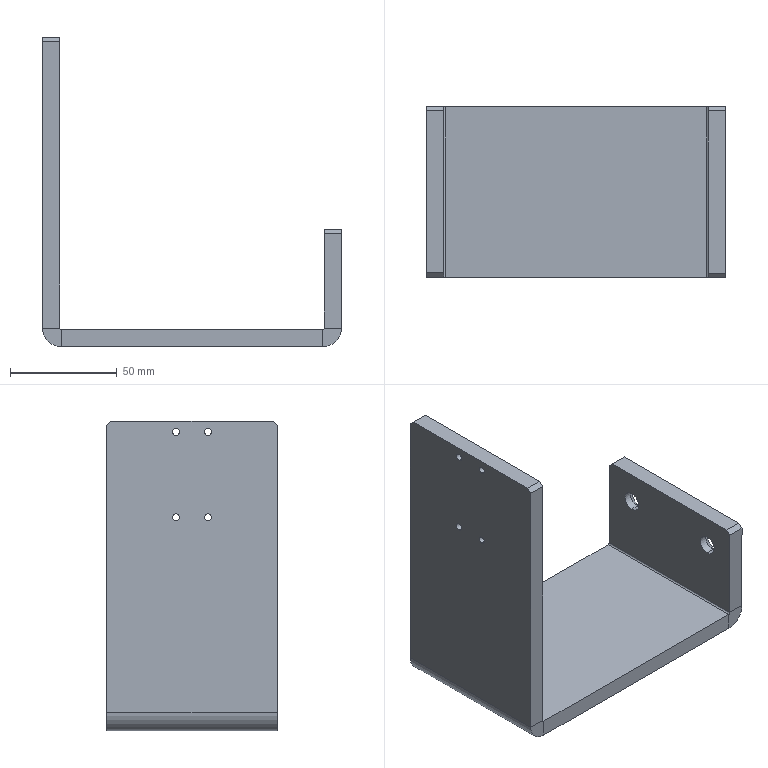Part | SolidWorks | features EdgeFlange 2, HoleWzd 2, Chamfer 1, FlatPattern 1, SMBaseFlange 1, SheetMetal 1 | 1 solid | 42 faces | box 140 x 80 x 145 mm | volume 202654 mm3 | plane 22 | cylinder 16 | cone 4 | commonest cylinder face diameters 3.3 x8 9 x4 1.473 x2 17.473 x2
STEP:
#1=CARTESIAN_POINT('',(-62.,7.5,133.65));
#2=VERTEX_POINT('',#1);
#3=CARTESIAN_POINT('',(-62.,7.5,130.35));
#4=VERTEX_POINT('',#3);
#5=CARTESIAN_POINT('',(-62.,7.5,132.));
#6=DIRECTION('',(1.,0.,0.));
#7=DIRECTION('',(0.,0.,-1.));
#8=AXIS2_PLACEMENT_3D('',#5,#6,#7);
#9=CIRCLE('',#8,1.65);
#10=EDGE_CURVE('',#2,#4,#9,.T.);
#11=ORIENTED_EDGE('',*,*,#10,.T.);
#12=CARTESIAN_POINT('',(-70.,7.5,130.35));
#13=VERTEX_POINT('',#12);
#14=CARTESIAN_POINT('',(-70.,7.5,130.35));
#15=DIRECTION('',(-1.,0.,0.));
#16=VECTOR('',#15,1000.);
#17=LINE('',#14,#16);
#18=EDGE_CURVE('',#4,#13,#17,.T.);
#19=ORIENTED_EDGE('',*,*,#18,.T.);
#20=CARTESIAN_POINT('',(-70.,7.5,133.65));
#21=VERTEX_POINT('',#20);
#22=CARTESIAN_POINT('',(-70.,7.5,132.));
#23=DIRECTION('',(-1.,0.,0.));
#24=DIRECTION('',(0.,0.,1.));
#25=AXIS2_PLACEMENT_3D('',#22,#23,#24);
#26=CIRCLE('',#25,1.65);
#27=EDGE_CURVE('',#13,#21,#26,.T.);
#28=ORIENTED_EDGE('',*,*,#27,.T.);
#29=CARTESIAN_POINT('',(-70.,7.5,133.65));
#30=DIRECTION('',(-1.,0.,0.));
#31=VECTOR('',#30,1000.);
#32=LINE('',#29,#31);
#33=EDGE_CURVE('',#2,#21,#32,.T.);
#34=ORIENTED_EDGE('',*,*,#33,.F.);
#35=EDGE_LOOP('',(#11,#19,#28,#34));
#36=FACE_OUTER_BOUND('',#35,.T.);
#37=CARTESIAN_POINT('',(-70.,7.5,132.));
#38=DIRECTION('',(-1.,0.,0.));
#39=DIRECTION('',(0.,0.,1.));
#40=AXIS2_PLACEMENT_3D('',#37,#38,#39);
#41=CYLINDRICAL_SURFACE('',#40,1.65);
#42=ADVANCED_FACE('',(#36),#41,.F.);
#43=CARTESIAN_POINT('',(-62.,-7.5,133.65));
#44=VERTEX_POINT('',#43);
#45=CARTESIAN_POINT('',(-62.,-7.5,130.35));
#46=VERTEX_POINT('',#45);
#47=CARTESIAN_POINT('',(-62.,-7.5,132.));
#48=DIRECTION('',(1.,0.,0.));
#49=DIRECTION('',(0.,0.,-1.));
#50=AXIS2_PLACEMENT_3D('',#47,#48,#49);
#51=CIRCLE('',#50,1.65);
#52=EDGE_CURVE('',#44,#46,#51,.T.);
#53=ORIENTED_EDGE('',*,*,#52,.T.);
#54=CARTESIAN_POINT('',(-70.,-7.5,130.35));
#55=VERTEX_POINT('',#54);
#56=CARTESIAN_POINT('',(-70.,-7.5,130.35));
#57=DIRECTION('',(-1.,0.,0.));
#58=VECTOR('',#57,1000.);
#59=LINE('',#56,#58);
#60=EDGE_CURVE('',#46,#55,#59,.T.);
#61=ORIENTED_EDGE('',*,*,#60,.T.);
#62=CARTESIAN_POINT('',(-70.,-7.5,133.65));
#63=VERTEX_POINT('',#62);
#64=CARTESIAN_POINT('',(-70.,-7.5,132.));
#65=DIRECTION('',(-1.,0.,0.));
#66=DIRECTION('',(0.,0.,1.));
#67=AXIS2_PLACEMENT_3D('',#64,#65,#66);
#68=CIRCLE('',#67,1.65);
#69=EDGE_CURVE('',#55,#63,#68,.T.);
#70=ORIENTED_EDGE('',*,*,#69,.T.);
#71=CARTESIAN_POINT('',(-70.,-7.5,133.65));
#72=DIRECTION('',(-1.,0.,0.));
#73=VECTOR('',#72,1000.);
#74=LINE('',#71,#73);
#75=EDGE_CURVE('',#44,#63,#74,.T.);
#76=ORIENTED_EDGE('',*,*,#75,.F.);
#77=EDGE_LOOP('',(#53,#61,#70,#76));
#78=FACE_OUTER_BOUND('',#77,.T.);
#79=CARTESIAN_POINT('',(-70.,-7.5,132.));
#80=DIRECTION('',(-1.,0.,0.));
#81=DIRECTION('',(0.,0.,1.));
#82=AXIS2_PLACEMENT_3D('',#79,#80,#81);
#83=CYLINDRICAL_SURFACE('',#82,1.65);
#84=ADVANCED_FACE('',(#78),#83,.F.);
#85=CARTESIAN_POINT('',(-62.,-7.5,93.65));
#86=VERTEX_POINT('',#85);
#87=CARTESIAN_POINT('',(-62.,-7.5,90.35));
#88=VERTEX_POINT('',#87);
#89=CARTESIAN_POINT('',(-62.,-7.5,92.));
#90=DIRECTION('',(1.,0.,0.));
#91=DIRECTION('',(0.,0.,-1.));
#92=AXIS2_PLACEMENT_3D('',#89,#90,#91);
#93=CIRCLE('',#92,1.65);
#94=EDGE_CURVE('',#86,#88,#93,.T.);
#95=ORIENTED_EDGE('',*,*,#94,.T.);
#96=CARTESIAN_POINT('',(-70.,-7.5,90.35));
#97=VERTEX_POINT('',#96);
#98=CARTESIAN_POINT('',(-70.,-7.5,90.35));
#99=DIRECTION('',(-1.,0.,0.));
#100=VECTOR('',#99,1000.);
#101=LINE('',#98,#100);
#102=EDGE_CURVE('',#88,#97,#101,.T.);
#103=ORIENTED_EDGE('',*,*,#102,.T.);
#104=CARTESIAN_POINT('',(-70.,-7.5,93.65));
#105=VERTEX_POINT('',#104);
#106=CARTESIAN_POINT('',(-70.,-7.5,92.));
#107=DIRECTION('',(-1.,0.,0.));
#108=DIRECTION('',(0.,0.,1.));
#109=AXIS2_PLACEMENT_3D('',#106,#107,#108);
#110=CIRCLE('',#109,1.65);
#111=EDGE_CURVE('',#97,#105,#110,.T.);
#112=ORIENTED_EDGE('',*,*,#111,.T.);
#113=CARTESIAN_POINT('',(-70.,-7.5,93.65));
#114=DIRECTION('',(-1.,0.,0.));
#115=VECTOR('',#114,1000.);
#116=LINE('',#113,#115);
#117=EDGE_CURVE('',#86,#105,#116,.T.);
#118=ORIENTED_EDGE('',*,*,#117,.F.);
#119=EDGE_LOOP('',(#95,#103,#112,#118));
#120=FACE_OUTER_BOUND('',#119,.T.);
#121=CARTESIAN_POINT('',(-70.,-7.5,92.));
#122=DIRECTION('',(-1.,0.,0.));
#123=DIRECTION('',(0.,0.,1.));
#124=AXIS2_PLACEMENT_3D('',#121,#122,#123);
#125=CYLINDRICAL_SURFACE('',#124,1.65);
#126=ADVANCED_FACE('',(#120),#125,.F.);
#127=CARTESIAN_POINT('',(-62.,7.5,93.65));
#128=VERTEX_POINT('',#127);
#129=CARTESIAN_POINT('',(-62.,7.5,90.35));
#130=VERTEX_POINT('',#129);
#131=CARTESIAN_POINT('',(-62.,7.5,92.));
#132=DIRECTION('',(1.,0.,0.));
#133=DIRECTION('',(0.,0.,-1.));
#134=AXIS2_PLACEMENT_3D('',#131,#132,#133);
#135=CIRCLE('',#134,1.65);
#136=EDGE_CURVE('',#128,#130,#135,.T.);
#137=ORIENTED_EDGE('',*,*,#136,.T.);
#138=CARTESIAN_POINT('',(-70.,7.5,90.35));
#139=VERTEX_POINT('',#138);
#140=CARTESIAN_POINT('',(-70.,7.5,90.35));
#141=DIRECTION('',(-1.,0.,0.));
#142=VECTOR('',#141,1000.);
#143=LINE('',#140,#142);
#144=EDGE_CURVE('',#130,#139,#143,.T.);
#145=ORIENTED_EDGE('',*,*,#144,.T.);
#146=CARTESIAN_POINT('',(-70.,7.5,93.65));
#147=VERTEX_POINT('',#146);
#148=CARTESIAN_POINT('',(-70.,7.5,92.));
#149=DIRECTION('',(-1.,0.,0.));
#150=DIRECTION('',(0.,0.,1.));
#151=AXIS2_PLACEMENT_3D('',#148,#149,#150);
#152=CIRCLE('',#151,1.65);
#153=EDGE_CURVE('',#139,#147,#152,.T.);
#154=ORIENTED_EDGE('',*,*,#153,.T.);
#155=CARTESIAN_POINT('',(-70.,7.5,93.65));
#156=DIRECTION('',(-1.,0.,0.));
#157=VECTOR('',#156,1000.);
#158=LINE('',#155,#157);
#159=EDGE_CURVE('',#128,#147,#158,.T.);
#160=ORIENTED_EDGE('',*,*,#159,.F.);
#161=EDGE_LOOP('',(#137,#145,#154,#160));
#162=FACE_OUTER_BOUND('',#161,.T.);
#163=CARTESIAN_POINT('',(-70.,7.5,92.));
#164=DIRECTION('',(-1.,0.,0.));
#165=DIRECTION('',(0.,0.,1.));
#166=AXIS2_PLACEMENT_3D('',#163,#164,#165);
#167=CYLINDRICAL_SURFACE('',#166,1.65);
#168=ADVANCED_FACE('',(#162),#167,.F.);
#169=CARTESIAN_POINT('',(65.54,-25.,36.5));
#170=VERTEX_POINT('',#169);
#171=CARTESIAN_POINT('',(65.54,-25.,27.5));
#172=VERTEX_POINT('',#171);
#173=CARTESIAN_POINT('',(65.54,-25.,32.));
#174=DIRECTION('',(1.,0.,0.));
#175=DIRECTION('',(0.,0.,-1.));
#176=AXIS2_PLACEMENT_3D('',#173,#174,#175);
#177=CIRCLE('',#176,4.5);
#178=EDGE_CURVE('',#170,#172,#177,.T.);
#179=ORIENTED_EDGE('',*,*,#178,.F.);
#180=CARTESIAN_POINT('',(70.,-25.,40.96));
#181=VERTEX_POINT('',#180);
#182=CARTESIAN_POINT('',(70.,-25.,40.96));
#183=DIRECTION('',(0.7071,0.,0.7071));
#184=VECTOR('',#183,1000.);
#185=LINE('',#182,#184);
#186=EDGE_CURVE('',#170,#181,#185,.T.);
#187=ORIENTED_EDGE('',*,*,#186,.T.);
#188=CARTESIAN_POINT('',(70.,-25.,23.04));
#189=VERTEX_POINT('',#188);
#190=CARTESIAN_POINT('',(70.,-25.,32.));
#191=DIRECTION('',(1.,0.,0.));
#192=DIRECTION('',(0.,0.,-1.));
#193=AXIS2_PLACEMENT_3D('',#190,#191,#192);
#194=CIRCLE('',#193,8.96);
#195=EDGE_CURVE('',#181,#189,#194,.T.);
#196=ORIENTED_EDGE('',*,*,#195,.T.);
#197=CARTESIAN_POINT('',(70.,-25.,23.04));
#198=DIRECTION('',(0.7071,0.,-0.7071));
#199=VECTOR('',#198,1000.);
#200=LINE('',#197,#199);
#201=EDGE_CURVE('',#172,#189,#200,.T.);
#202=ORIENTED_EDGE('',*,*,#201,.F.);
#203=EDGE_LOOP('',(#179,#187,#196,#202));
#204=FACE_OUTER_BOUND('',#203,.T.);
#205=CARTESIAN_POINT('',(70.,-25.,32.));
#206=DIRECTION('',(1.,0.,0.));
#207=DIRECTION('',(0.,0.,-1.));
#208=AXIS2_PLACEMENT_3D('',#205,#206,#207);
#209=CONICAL_SURFACE('',#208,8.96,0.7854);
#210=ADVANCED_FACE('',(#204),#209,.F.);
#211=CARTESIAN_POINT('',(62.,-25.,27.5));
#212=VERTEX_POINT('',#211);
#213=CARTESIAN_POINT('',(62.,-25.,36.5));
#214=VERTEX_POINT('',#213);
#215=CARTESIAN_POINT('',(62.,-25.,32.));
#216=DIRECTION('',(-1.,0.,0.));
#217=DIRECTION('',(0.,0.,1.));
#218=AXIS2_PLACEMENT_3D('',#215,#216,#217);
#219=CIRCLE('',#218,4.5);
#220=EDGE_CURVE('',#212,#214,#219,.T.);
#221=ORIENTED_EDGE('',*,*,#220,.T.);
#222=CARTESIAN_POINT('',(70.,-25.,36.5));
#223=DIRECTION('',(1.,0.,0.));
#224=VECTOR('',#223,1000.);
#225=LINE('',#222,#224);
#226=EDGE_CURVE('',#214,#170,#225,.T.);
#227=ORIENTED_EDGE('',*,*,#226,.T.);
#228=ORIENTED_EDGE('',*,*,#178,.T.);
#229=CARTESIAN_POINT('',(70.,-25.,27.5));
#230=DIRECTION('',(1.,0.,0.));
#231=VECTOR('',#230,1000.);
#232=LINE('',#229,#231);
#233=EDGE_CURVE('',#212,#172,#232,.T.);
#234=ORIENTED_EDGE('',*,*,#233,.F.);
#235=EDGE_LOOP('',(#221,#227,#228,#234));
#236=FACE_OUTER_BOUND('',#235,.T.);
#237=CARTESIAN_POINT('',(70.,-25.,32.));
#238=DIRECTION('',(1.,0.,0.));
#239=DIRECTION('',(0.,0.,-1.));
#240=AXIS2_PLACEMENT_3D('',#237,#238,#239);
#241=CYLINDRICAL_SURFACE('',#240,4.5);
#242=ADVANCED_FACE('',(#236),#241,.F.);
#243=CARTESIAN_POINT('',(65.54,25.,36.5));
#244=VERTEX_POINT('',#243);
#245=CARTESIAN_POINT('',(65.54,25.,27.5));
#246=VERTEX_POINT('',#245);
#247=CARTESIAN_POINT('',(65.54,25.,32.));
#248=DIRECTION('',(1.,0.,0.));
#249=DIRECTION('',(0.,0.,-1.));
#250=AXIS2_PLACEMENT_3D('',#247,#248,#249);
#251=CIRCLE('',#250,4.5);
#252=EDGE_CURVE('',#244,#246,#251,.T.);
#253=ORIENTED_EDGE('',*,*,#252,.F.);
#254=CARTESIAN_POINT('',(70.,25.,40.96));
#255=VERTEX_POINT('',#254);
#256=CARTESIAN_POINT('',(70.,25.,40.96));
#257=DIRECTION('',(0.7071,0.,0.7071));
#258=VECTOR('',#257,1000.);
#259=LINE('',#256,#258);
#260=EDGE_CURVE('',#244,#255,#259,.T.);
#261=ORIENTED_EDGE('',*,*,#260,.T.);
#262=CARTESIAN_POINT('',(70.,25.,23.04));
#263=VERTEX_POINT('',#262);
#264=CARTESIAN_POINT('',(70.,25.,32.));
#265=DIRECTION('',(1.,0.,0.));
#266=DIRECTION('',(0.,0.,-1.));
#267=AXIS2_PLACEMENT_3D('',#264,#265,#266);
#268=CIRCLE('',#267,8.96);
#269=EDGE_CURVE('',#255,#263,#268,.T.);
#270=ORIENTED_EDGE('',*,*,#269,.T.);
#271=CARTESIAN_POINT('',(70.,25.,23.04));
#272=DIRECTION('',(0.7071,0.,-0.7071));
#273=VECTOR('',#272,1000.);
#274=LINE('',#271,#273);
#275=EDGE_CURVE('',#246,#263,#274,.T.);
#276=ORIENTED_EDGE('',*,*,#275,.F.);
#277=EDGE_LOOP('',(#253,#261,#270,#276));
#278=FACE_OUTER_BOUND('',#277,.T.);
#279=CARTESIAN_POINT('',(70.,25.,32.));
#280=DIRECTION('',(1.,0.,0.));
#281=DIRECTION('',(0.,0.,-1.));
#282=AXIS2_PLACEMENT_3D('',#279,#280,#281);
#283=CONICAL_SURFACE('',#282,8.96,0.7854);
#284=ADVANCED_FACE('',(#278),#283,.F.);
#285=CARTESIAN_POINT('',(62.,25.,27.5));
#286=VERTEX_POINT('',#285);
#287=CARTESIAN_POINT('',(62.,25.,36.5));
#288=VERTEX_POINT('',#287);
#289=CARTESIAN_POINT('',(62.,25.,32.));
#290=DIRECTION('',(-1.,0.,0.));
#291=DIRECTION('',(0.,0.,1.));
#292=AXIS2_PLACEMENT_3D('',#289,#290,#291);
#293=CIRCLE('',#292,4.5);
#294=EDGE_CURVE('',#286,#288,#293,.T.);
#295=ORIENTED_EDGE('',*,*,#294,.T.);
#296=CARTESIAN_POINT('',(70.,25.,36.5));
#297=DIRECTION('',(1.,0.,0.));
#298=VECTOR('',#297,1000.);
#299=LINE('',#296,#298);
#300=EDGE_CURVE('',#288,#244,#299,.T.);
#301=ORIENTED_EDGE('',*,*,#300,.T.);
#302=ORIENTED_EDGE('',*,*,#252,.T.);
#303=CARTESIAN_POINT('',(70.,25.,27.5));
#304=DIRECTION('',(1.,0.,0.));
#305=VECTOR('',#304,1000.);
#306=LINE('',#303,#305);
#307=EDGE_CURVE('',#286,#246,#306,.T.);
#308=ORIENTED_EDGE('',*,*,#307,.F.);
#309=EDGE_LOOP('',(#295,#301,#302,#308));
#310=FACE_OUTER_BOUND('',#309,.T.);
#311=CARTESIAN_POINT('',(70.,25.,32.));
#312=DIRECTION('',(1.,0.,0.));
#313=DIRECTION('',(0.,0.,-1.));
#314=AXIS2_PLACEMENT_3D('',#311,#312,#313);
#315=CYLINDRICAL_SURFACE('',#314,4.5);
#316=ADVANCED_FACE('',(#310),#315,.F.);
#317=CARTESIAN_POINT('',(-70.,7.5,132.));
#318=DIRECTION('',(-1.,0.,0.));
#319=DIRECTION('',(0.,0.,1.));
#320=AXIS2_PLACEMENT_3D('',#317,#318,#319);
#321=CIRCLE('',#320,1.65);
#322=EDGE_CURVE('',#21,#13,#321,.T.);
#323=ORIENTED_EDGE('',*,*,#322,.F.);
#324=ORIENTED_EDGE('',*,*,#27,.F.);
#325=EDGE_LOOP('',(#323,#324));
#326=FACE_BOUND('',#325,.T.);
#327=CARTESIAN_POINT('',(-70.,-7.5,132.));
#328=DIRECTION('',(-1.,0.,0.));
#329=DIRECTION('',(0.,0.,1.));
#330=AXIS2_PLACEMENT_3D('',#327,#328,#329);
#331=CIRCLE('',#330,1.65);
#332=EDGE_CURVE('',#63,#55,#331,.T.);
#333=ORIENTED_EDGE('',*,*,#332,.F.);
#334=ORIENTED_EDGE('',*,*,#69,.F.);
#335=EDGE_LOOP('',(#333,#334));
#336=FACE_BOUND('',#335,.T.);
#337=CARTESIAN_POINT('',(-70.,7.5,92.));
#338=DIRECTION('',(-1.,0.,0.));
#339=DIRECTION('',(0.,0.,1.));
#340=AXIS2_PLACEMENT_3D('',#337,#338,#339);
#341=CIRCLE('',#340,1.65);
#342=EDGE_CURVE('',#147,#139,#341,.T.);
#343=ORIENTED_EDGE('',*,*,#342,.F.);
#344=ORIENTED_EDGE('',*,*,#153,.F.);
#345=EDGE_LOOP('',(#343,#344));
#346=FACE_BOUND('',#345,.T.);
#347=CARTESIAN_POINT('',(-70.,-38.,137.));
#348=VERTEX_POINT('',#347);
#349=CARTESIAN_POINT('',(-70.,38.,137.));
#350=VERTEX_POINT('',#349);
#351=CARTESIAN_POINT('',(-70.,0.,137.));
#352=DIRECTION('',(0.,1.,0.));
#353=VECTOR('',#352,1000.);
#354=LINE('',#351,#353);
#355=EDGE_CURVE('',#348,#350,#354,.T.);
#356=ORIENTED_EDGE('',*,*,#355,.T.);
#357=CARTESIAN_POINT('',(-70.,40.,135.));
#358=VERTEX_POINT('',#357);
#359=CARTESIAN_POINT('',(-70.,40.,135.));
#360=DIRECTION('',(0.,0.7071,-0.7071));
#361=VECTOR('',#360,1000.);
#362=LINE('',#359,#361);
#363=EDGE_CURVE('',#350,#358,#362,.T.);
#364=ORIENTED_EDGE('',*,*,#363,.T.);
#365=CARTESIAN_POINT('',(-70.,40.,0.7366));
#366=VERTEX_POINT('',#365);
#367=CARTESIAN_POINT('',(-70.,40.,0.));
#368=DIRECTION('',(0.,0.,-1.));
#369=VECTOR('',#368,1000.);
#370=LINE('',#367,#369);
#371=EDGE_CURVE('',#358,#366,#370,.T.);
#372=ORIENTED_EDGE('',*,*,#371,.T.);
#373=CARTESIAN_POINT('',(-70.,-40.,0.7366));
#374=VERTEX_POINT('',#373);
#375=CARTESIAN_POINT('',(-70.,40.,0.7366));
#376=DIRECTION('',(0.,1.,0.));
#377=VECTOR('',#376,1000.);
#378=LINE('',#375,#377);
#379=EDGE_CURVE('',#374,#366,#378,.T.);
#380=ORIENTED_EDGE('',*,*,#379,.F.);
#381=CARTESIAN_POINT('',(-70.,-40.,135.));
#382=VERTEX_POINT('',#381);
#383=CARTESIAN_POINT('',(-70.,-40.,0.));
#384=DIRECTION('',(0.,0.,1.));
#385=VECTOR('',#384,1000.);
#386=LINE('',#383,#385);
#387=EDGE_CURVE('',#374,#382,#386,.T.);
#388=ORIENTED_EDGE('',*,*,#387,.T.);
#389=CARTESIAN_POINT('',(-70.,-38.,137.));
#390=DIRECTION('',(0.,0.7071,0.7071));
#391=VECTOR('',#390,1000.);
#392=LINE('',#389,#391);
#393=EDGE_CURVE('',#382,#348,#392,.T.);
#394=ORIENTED_EDGE('',*,*,#393,.T.);
#395=EDGE_LOOP('',(#356,#364,#372,#380,#388,#394));
#396=FACE_OUTER_BOUND('',#395,.T.);
#397=CARTESIAN_POINT('',(-70.,-7.5,92.));
#398=DIRECTION('',(-1.,0.,0.));
#399=DIRECTION('',(0.,0.,1.));
#400=AXIS2_PLACEMENT_3D('',#397,#398,#399);
#401=CIRCLE('',#400,1.65);
#402=EDGE_CURVE('',#105,#97,#401,.T.);
#403=ORIENTED_EDGE('',*,*,#402,.F.);
#404=ORIENTED_EDGE('',*,*,#111,.F.);
#405=EDGE_LOOP('',(#403,#404));
#406=FACE_BOUND('',#405,.T.);
#407=CARTESIAN_POINT('',(-70.,0.,0.));
#408=DIRECTION('',(1.,0.,0.));
#409=DIRECTION('',(0.,0.,-1.));
#410=AXIS2_PLACEMENT_3D('',#407,#408,#409);
#411=PLANE('',#410);
#412=ADVANCED_FACE('',(#326,#336,#346,#396,#406),#411,.F.);
#413=CARTESIAN_POINT('',(61.263,40.,-8.));
#414=VERTEX_POINT('',#413);
#415=CARTESIAN_POINT('',(61.263,-40.,-8.));
#416=VERTEX_POINT('',#415);
#417=CARTESIAN_POINT('',(61.263,40.,-8.));
#418=DIRECTION('',(0.,-1.,0.));
#419=VECTOR('',#418,1000.);
#420=LINE('',#417,#419);
#421=EDGE_CURVE('',#414,#416,#420,.T.);
#422=ORIENTED_EDGE('',*,*,#421,.T.);
#423=CARTESIAN_POINT('',(-61.263,-40.,-8.));
#424=VERTEX_POINT('',#423);
#425=CARTESIAN_POINT('',(-70.,-40.,-8.));
#426=DIRECTION('',(1.,0.,0.));
#427=VECTOR('',#426,1000.);
#428=LINE('',#425,#427);
#429=EDGE_CURVE('',#424,#416,#428,.T.);
#430=ORIENTED_EDGE('',*,*,#429,.F.);
#431=CARTESIAN_POINT('',(-61.263,40.,-8.));
#432=VERTEX_POINT('',#431);
#433=CARTESIAN_POINT('',(-61.263,-40.,-8.));
#434=DIRECTION('',(0.,1.,0.));
#435=VECTOR('',#434,1000.);
#436=LINE('',#433,#435);
#437=EDGE_CURVE('',#424,#432,#436,.T.);
#438=ORIENTED_EDGE('',*,*,#437,.T.);
#439=CARTESIAN_POINT('',(-70.,40.,-8.));
#440=DIRECTION('',(-1.,0.,0.));
#441=VECTOR('',#440,1000.);
#442=LINE('',#439,#441);
#443=EDGE_CURVE('',#414,#432,#442,.T.);
#444=ORIENTED_EDGE('',*,*,#443,.F.);
#445=EDGE_LOOP('',(#422,#430,#438,#444));
#446=FACE_OUTER_BOUND('',#445,.T.);
#447=CARTESIAN_POINT('',(0.,0.,-8.));
#448=DIRECTION('',(0.,0.,1.));
#449=DIRECTION('',(1.,0.,0.));
#450=AXIS2_PLACEMENT_3D('',#447,#448,#449);
#451=PLANE('',#450);
#452=ADVANCED_FACE('',(#446),#451,.F.);
#453=CARTESIAN_POINT('',(-61.263,-40.,0.));
#454=VERTEX_POINT('',#453);
#455=CARTESIAN_POINT('',(61.263,-40.,0.));
#456=VERTEX_POINT('',#455);
#457=CARTESIAN_POINT('',(-70.,-40.,0.));
#458=DIRECTION('',(1.,0.,0.));
#459=VECTOR('',#458,1000.);
#460=LINE('',#457,#459);
#461=EDGE_CURVE('',#454,#456,#460,.T.);
#462=ORIENTED_EDGE('',*,*,#461,.T.);
#463=CARTESIAN_POINT('',(61.263,40.,0.));
#464=VERTEX_POINT('',#463);
#465=CARTESIAN_POINT('',(61.263,40.,0.));
#466=DIRECTION('',(0.,-1.,0.));
#467=VECTOR('',#466,1000.);
#468=LINE('',#465,#467);
#469=EDGE_CURVE('',#464,#456,#468,.T.);
#470=ORIENTED_EDGE('',*,*,#469,.F.);
#471=CARTESIAN_POINT('',(-61.263,40.,0.));
#472=VERTEX_POINT('',#471);
#473=CARTESIAN_POINT('',(-70.,40.,0.));
#474=DIRECTION('',(-1.,0.,0.));
#475=VECTOR('',#474,1000.);
#476=LINE('',#473,#475);
#477=EDGE_CURVE('',#464,#472,#476,.T.);
#478=ORIENTED_EDGE('',*,*,#477,.T.);
#479=CARTESIAN_POINT('',(-61.263,-40.,0.));
#480=DIRECTION('',(0.,1.,0.));
#481=VECTOR('',#480,1000.);
#482=LINE('',#479,#481);
#483=EDGE_CURVE('',#454,#472,#482,.T.);
#484=ORIENTED_EDGE('',*,*,#483,.F.);
#485=EDGE_LOOP('',(#462,#470,#478,#484));
#486=FACE_OUTER_BOUND('',#485,.T.);
#487=CARTESIAN_POINT('',(0.,0.,0.));
#488=DIRECTION('',(0.,0.,1.));
#489=DIRECTION('',(1.,0.,0.));
#490=AXIS2_PLACEMENT_3D('',#487,#488,#489);
#491=PLANE('',#490);
#492=ADVANCED_FACE('',(#486),#491,.T.);
#493=ORIENTED_EDGE('',*,*,#477,.F.);
#494=CARTESIAN_POINT('',(61.263,40.,0.));
#495=DIRECTION('',(0.,0.,-1.));
#496=VECTOR('',#495,1000.);
#497=LINE('',#494,#496);
#498=EDGE_CURVE('',#464,#414,#497,.T.);
#499=ORIENTED_EDGE('',*,*,#498,.T.);
#500=ORIENTED_EDGE('',*,*,#443,.T.);
#501=CARTESIAN_POINT('',(-61.263,40.,0.));
#502=DIRECTION('',(0.,0.,-1.));
#503=VECTOR('',#502,1000.);
#504=LINE('',#501,#503);
#505=EDGE_CURVE('',#472,#432,#504,.T.);
#506=ORIENTED_EDGE('',*,*,#505,.F.);
#507=EDGE_LOOP('',(#493,#499,#500,#506));
#508=FACE_OUTER_BOUND('',#507,.T.);
#509=CARTESIAN_POINT('',(-70.,40.,-8.));
#510=DIRECTION('',(0.,1.,0.));
#511=DIRECTION('',(0.,0.,1.));
#512=AXIS2_PLACEMENT_3D('',#509,#510,#511);
#513=PLANE('',#512);
#514=ADVANCED_FACE('',(#508),#513,.T.);
#515=CARTESIAN_POINT('',(61.263,-40.,0.));
#516=DIRECTION('',(0.,0.,-1.));
#517=VECTOR('',#516,1000.);
#518=LINE('',#515,#517);
#519=EDGE_CURVE('',#456,#416,#518,.T.);
#520=ORIENTED_EDGE('',*,*,#519,.F.);
#521=ORIENTED_EDGE('',*,*,#461,.F.);
#522=CARTESIAN_POINT('',(-61.263,-40.,0.));
#523=DIRECTION('',(0.,0.,-1.));
#524=VECTOR('',#523,1000.);
#525=LINE('',#522,#524);
#526=EDGE_CURVE('',#454,#424,#525,.T.);
#527=ORIENTED_EDGE('',*,*,#526,.T.);
#528=ORIENTED_EDGE('',*,*,#429,.T.);
#529=EDGE_LOOP('',(#520,#521,#527,#528));
#530=FACE_OUTER_BOUND('',#529,.T.);
#531=CARTESIAN_POINT('',(-70.,-40.,-8.));
#532=DIRECTION('',(0.,-1.,0.));
#533=DIRECTION('',(0.,0.,-1.));
#534=AXIS2_PLACEMENT_3D('',#531,#532,#533);
#535=PLANE('',#534);
#536=ADVANCED_FACE('',(#530),#535,.T.);
#537=CARTESIAN_POINT('',(-62.,40.,0.7366));
#538=VERTEX_POINT('',#537);
#539=CARTESIAN_POINT('',(-70.,40.,0.7366));
#540=DIRECTION('',(-1.,0.,0.));
#541=VECTOR('',#540,1000.);
#542=LINE('',#539,#541);
#543=EDGE_CURVE('',#538,#366,#542,.T.);
#544=ORIENTED_EDGE('',*,*,#543,.F.);
#545=CARTESIAN_POINT('',(-61.263,40.,0.7366));
#546=DIRECTION('',(0.,1.,0.));
#547=DIRECTION('',(0.,0.,-1.));
#548=AXIS2_PLACEMENT_3D('',#545,#546,#547);
#549=CIRCLE('',#548,0.7366);
#550=EDGE_CURVE('',#472,#538,#549,.T.);
#551=ORIENTED_EDGE('',*,*,#550,.F.);
#552=ORIENTED_EDGE('',*,*,#505,.T.);
#553=CARTESIAN_POINT('',(-61.263,40.,0.7366));
#554=DIRECTION('',(0.,1.,0.));
#555=DIRECTION('',(0.,0.,-1.));
#556=AXIS2_PLACEMENT_3D('',#553,#554,#555);
#557=CIRCLE('',#556,8.737);
#558=EDGE_CURVE('',#432,#366,#557,.T.);
#559=ORIENTED_EDGE('',*,*,#558,.T.);
#560=EDGE_LOOP('',(#544,#551,#552,#559));
#561=FACE_OUTER_BOUND('',#560,.T.);
#562=CARTESIAN_POINT('',(-61.263,40.,0.7366));
#563=DIRECTION('',(0.,1.,0.));
#564=DIRECTION('',(0.,0.,1.));
#565=AXIS2_PLACEMENT_3D('',#562,#563,#564);
#566=PLANE('',#565);
#567=ADVANCED_FACE('',(#561),#566,.T.);
#568=CARTESIAN_POINT('',(-62.,-40.,0.7366));
#569=VERTEX_POINT('',#568);
#570=CARTESIAN_POINT('',(-61.263,-40.,0.7366));
#571=DIRECTION('',(0.,-1.,0.));
#572=DIRECTION('',(0.,0.,-1.));
#573=AXIS2_PLACEMENT_3D('',#570,#571,#572);
#574=CIRCLE('',#573,0.7366);
#575=EDGE_CURVE('',#569,#454,#574,.T.);
#576=ORIENTED_EDGE('',*,*,#575,.F.);
#577=CARTESIAN_POINT('',(-62.,-40.,0.7366));
#578=DIRECTION('',(-1.,0.,0.));
#579=VECTOR('',#578,1000.);
#580=LINE('',#577,#579);
#581=EDGE_CURVE('',#569,#374,#580,.T.);
#582=ORIENTED_EDGE('',*,*,#581,.T.);
#583=CARTESIAN_POINT('',(-61.263,-40.,0.7366));
#584=DIRECTION('',(0.,-1.,0.));
#585=DIRECTION('',(0.,0.,-1.));
#586=AXIS2_PLACEMENT_3D('',#583,#584,#585);
#587=CIRCLE('',#586,8.737);
#588=EDGE_CURVE('',#374,#424,#587,.T.);
#589=ORIENTED_EDGE('',*,*,#588,.T.);
#590=ORIENTED_EDGE('',*,*,#526,.F.);
#591=EDGE_LOOP('',(#576,#582,#589,#590));
#592=FACE_OUTER_BOUND('',#591,.T.);
#593=CARTESIAN_POINT('',(-61.263,-40.,0.7366));
#594=DIRECTION('',(0.,1.,0.));
#595=DIRECTION('',(0.,0.,1.));
#596=AXIS2_PLACEMENT_3D('',#593,#594,#595);
#597=PLANE('',#596);
#598=ADVANCED_FACE('',(#592),#597,.F.);
#599=ORIENTED_EDGE('',*,*,#437,.F.);
#600=ORIENTED_EDGE('',*,*,#588,.F.);
#601=ORIENTED_EDGE('',*,*,#379,.T.);
#602=ORIENTED_EDGE('',*,*,#558,.F.);
#603=EDGE_LOOP('',(#599,#600,#601,#602));
#604=FACE_OUTER_BOUND('',#603,.T.);
#605=CARTESIAN_POINT('',(-61.263,-40.,0.7366));
#606=DIRECTION('',(0.,-1.,0.));
#607=DIRECTION('',(-1.,0.,0.));
#608=AXIS2_PLACEMENT_3D('',#605,#606,#607);
#609=CYLINDRICAL_SURFACE('',#608,8.737);
#610=ADVANCED_FACE('',(#604),#609,.T.);
#611=ORIENTED_EDGE('',*,*,#483,.T.);
#612=ORIENTED_EDGE('',*,*,#550,.T.);
#613=CARTESIAN_POINT('',(-62.,40.,0.7366));
#614=DIRECTION('',(0.,-1.,0.));
#615=VECTOR('',#614,1000.);
#616=LINE('',#613,#615);
#617=EDGE_CURVE('',#538,#569,#616,.T.);
#618=ORIENTED_EDGE('',*,*,#617,.T.);
#619=ORIENTED_EDGE('',*,*,#575,.T.);
#620=EDGE_LOOP('',(#611,#612,#618,#619));
#621=FACE_OUTER_BOUND('',#620,.T.);
#622=CARTESIAN_POINT('',(-61.263,-40.,0.7366));
#623=DIRECTION('',(0.,-1.,0.));
#624=DIRECTION('',(-1.,0.,0.));
#625=AXIS2_PLACEMENT_3D('',#622,#623,#624);
#626=CYLINDRICAL_SURFACE('',#625,0.7366);
#627=ADVANCED_FACE('',(#621),#626,.F.);
#628=CARTESIAN_POINT('',(-62.,-40.,135.));
#629=VERTEX_POINT('',#628);
#630=CARTESIAN_POINT('',(-62.,-40.,137.));
#631=DIRECTION('',(0.,0.,1.));
#632=VECTOR('',#631,1000.);
#633=LINE('',#630,#632);
#634=EDGE_CURVE('',#569,#629,#633,.T.);
#635=ORIENTED_EDGE('',*,*,#634,.T.);
#636=CARTESIAN_POINT('',(-70.,-40.,135.));
#637=DIRECTION('',(-1.,0.,0.));
#638=VECTOR('',#637,1000.);
#639=LINE('',#636,#638);
#640=EDGE_CURVE('',#629,#382,#639,.T.);
#641=ORIENTED_EDGE('',*,*,#640,.T.);
#642=ORIENTED_EDGE('',*,*,#387,.F.);
#643=ORIENTED_EDGE('',*,*,#581,.F.);
#644=EDGE_LOOP('',(#635,#641,#642,#643));
#645=FACE_OUTER_BOUND('',#644,.T.);
#646=CARTESIAN_POINT('',(-70.,-40.,137.));
#647=DIRECTION('',(0.,1.,0.));
#648=DIRECTION('',(-1.,0.,0.));
#649=AXIS2_PLACEMENT_3D('',#646,#647,#648);
#650=PLANE('',#649);
#651=ADVANCED_FACE('',(#645),#650,.F.);
#652=ORIENTED_EDGE('',*,*,#371,.F.);
#653=CARTESIAN_POINT('',(-62.,40.,135.));
#654=VERTEX_POINT('',#653);
#655=CARTESIAN_POINT('',(-70.,40.,135.));
#656=DIRECTION('',(1.,0.,0.));
#657=VECTOR('',#656,1000.);
#658=LINE('',#655,#657);
#659=EDGE_CURVE('',#358,#654,#658,.T.);
#660=ORIENTED_EDGE('',*,*,#659,.T.);
#661=CARTESIAN_POINT('',(-62.,40.,0.));
#662=DIRECTION('',(0.,0.,-1.));
#663=VECTOR('',#662,1000.);
#664=LINE('',#661,#663);
#665=EDGE_CURVE('',#654,#538,#664,.T.);
#666=ORIENTED_EDGE('',*,*,#665,.T.);
#667=ORIENTED_EDGE('',*,*,#543,.T.);
#668=EDGE_LOOP('',(#652,#660,#666,#667));
#669=FACE_OUTER_BOUND('',#668,.T.);
#670=CARTESIAN_POINT('',(-70.,40.,0.));
#671=DIRECTION('',(0.,-1.,0.));
#672=DIRECTION('',(1.,0.,0.));
#673=AXIS2_PLACEMENT_3D('',#670,#671,#672);
#674=PLANE('',#673);
#675=ADVANCED_FACE('',(#669),#674,.F.);
#676=ORIENTED_EDGE('',*,*,#10,.F.);
#677=CARTESIAN_POINT('',(-62.,7.5,132.));
#678=DIRECTION('',(1.,0.,0.));
#679=DIRECTION('',(0.,0.,-1.));
#680=AXIS2_PLACEMENT_3D('',#677,#678,#679);
#681=CIRCLE('',#680,1.65);
#682=EDGE_CURVE('',#4,#2,#681,.T.);
#683=ORIENTED_EDGE('',*,*,#682,.F.);
#684=EDGE_LOOP('',(#676,#683));
#685=FACE_BOUND('',#684,.T.);
#686=ORIENTED_EDGE('',*,*,#52,.F.);
#687=CARTESIAN_POINT('',(-62.,-7.5,132.));
#688=DIRECTION('',(1.,0.,0.));
#689=DIRECTION('',(0.,0.,-1.));
#690=AXIS2_PLACEMENT_3D('',#687,#688,#689);
#691=CIRCLE('',#690,1.65);
#692=EDGE_CURVE('',#46,#44,#691,.T.);
#693=ORIENTED_EDGE('',*,*,#692,.F.);
#694=EDGE_LOOP('',(#686,#693));
#695=FACE_BOUND('',#694,.T.);
#696=ORIENTED_EDGE('',*,*,#94,.F.);
#697=CARTESIAN_POINT('',(-62.,-7.5,92.));
#698=DIRECTION('',(1.,0.,0.));
#699=DIRECTION('',(0.,0.,-1.));
#700=AXIS2_PLACEMENT_3D('',#697,#698,#699);
#701=CIRCLE('',#700,1.65);
#702=EDGE_CURVE('',#88,#86,#701,.T.);
#703=ORIENTED_EDGE('',*,*,#702,.F.);
#704=EDGE_LOOP('',(#696,#703));
#705=FACE_BOUND('',#704,.T.);
#706=ORIENTED_EDGE('',*,*,#136,.F.);
#707=CARTESIAN_POINT('',(-62.,7.5,92.));
#708=DIRECTION('',(1.,0.,0.));
#709=DIRECTION('',(0.,0.,-1.));
#710=AXIS2_PLACEMENT_3D('',#707,#708,#709);
#711=CIRCLE('',#710,1.65);
#712=EDGE_CURVE('',#130,#128,#711,.T.);
#713=ORIENTED_EDGE('',*,*,#712,.F.);
#714=EDGE_LOOP('',(#706,#713));
#715=FACE_BOUND('',#714,.T.);
#716=ORIENTED_EDGE('',*,*,#665,.F.);
#717=CARTESIAN_POINT('',(-62.,38.,137.));
#718=VERTEX_POINT('',#717);
#719=CARTESIAN_POINT('',(-62.,87.5,87.5));
#720=DIRECTION('',(0.,-0.7071,0.7071));
#721=VECTOR('',#720,1000.);
#722=LINE('',#719,#721);
#723=EDGE_CURVE('',#654,#718,#722,.T.);
#724=ORIENTED_EDGE('',*,*,#723,.T.);
#725=CARTESIAN_POINT('',(-62.,-38.,137.));
#726=VERTEX_POINT('',#725);
#727=CARTESIAN_POINT('',(-62.,40.,137.));
#728=DIRECTION('',(0.,1.,0.));
#729=VECTOR('',#728,1000.);
#730=LINE('',#727,#729);
#731=EDGE_CURVE('',#726,#718,#730,.T.);
#732=ORIENTED_EDGE('',*,*,#731,.F.);
#733=CARTESIAN_POINT('',(-62.,-87.5,87.5));
#734=DIRECTION('',(0.,-0.7071,-0.7071));
#735=VECTOR('',#734,1000.);
#736=LINE('',#733,#735);
#737=EDGE_CURVE('',#726,#629,#736,.T.);
#738=ORIENTED_EDGE('',*,*,#737,.T.);
#739=ORIENTED_EDGE('',*,*,#634,.F.);
#740=ORIENTED_EDGE('',*,*,#617,.F.);
#741=EDGE_LOOP('',(#716,#724,#732,#738,#739,#740));
#742=FACE_OUTER_BOUND('',#741,.T.);
#743=CARTESIAN_POINT('',(-62.,0.,0.));
#744=DIRECTION('',(1.,0.,0.));
#745=DIRECTION('',(0.,0.,-1.));
#746=AXIS2_PLACEMENT_3D('',#743,#744,#745);
#747=PLANE('',#746);
#748=ADVANCED_FACE('',(#685,#695,#705,#715,#742),#747,.T.);
#749=ORIENTED_EDGE('',*,*,#731,.T.);
#750=CARTESIAN_POINT('',(-70.,38.,137.));
#751=DIRECTION('',(-1.,0.,0.));
#752=VECTOR('',#751,1000.);
#753=LINE('',#750,#752);
#754=EDGE_CURVE('',#718,#350,#753,.T.);
#755=ORIENTED_EDGE('',*,*,#754,.T.);
#756=ORIENTED_EDGE('',*,*,#355,.F.);
#757=CARTESIAN_POINT('',(-70.,-38.,137.));
#758=DIRECTION('',(1.,0.,0.));
#759=VECTOR('',#758,1000.);
#760=LINE('',#757,#759);
#761=EDGE_CURVE('',#348,#726,#760,.T.);
#762=ORIENTED_EDGE('',*,*,#761,.T.);
#763=EDGE_LOOP('',(#749,#755,#756,#762));
#764=FACE_OUTER_BOUND('',#763,.T.);
#765=CARTESIAN_POINT('',(-70.,40.,137.));
#766=DIRECTION('',(0.,0.,-1.));
#767=DIRECTION('',(-1.,0.,0.));
#768=AXIS2_PLACEMENT_3D('',#765,#766,#767);
#769=PLANE('',#768);
#770=ADVANCED_FACE('',(#764),#769,.F.);
#771=CARTESIAN_POINT('',(62.,-40.,0.7366));
#772=VERTEX_POINT('',#771);
#773=CARTESIAN_POINT('',(70.,-40.,0.7366));
#774=VERTEX_POINT('',#773);
#775=CARTESIAN_POINT('',(70.,-40.,0.7366));
#776=DIRECTION('',(1.,0.,0.));
#777=VECTOR('',#776,1000.);
#778=LINE('',#775,#777);
#779=EDGE_CURVE('',#772,#774,#778,.T.);
#780=ORIENTED_EDGE('',*,*,#779,.F.);
#781=CARTESIAN_POINT('',(61.263,-40.,0.7366));
#782=DIRECTION('',(0.,-1.,0.));
#783=DIRECTION('',(0.,0.,1.));
#784=AXIS2_PLACEMENT_3D('',#781,#782,#783);
#785=CIRCLE('',#784,0.7366);
#786=EDGE_CURVE('',#456,#772,#785,.T.);
#787=ORIENTED_EDGE('',*,*,#786,.F.);
#788=ORIENTED_EDGE('',*,*,#519,.T.);
#789=CARTESIAN_POINT('',(61.263,-40.,0.7366));
#790=DIRECTION('',(0.,-1.,0.));
#791=DIRECTION('',(0.,0.,1.));
#792=AXIS2_PLACEMENT_3D('',#789,#790,#791);
#793=CIRCLE('',#792,8.737);
#794=EDGE_CURVE('',#416,#774,#793,.T.);
#795=ORIENTED_EDGE('',*,*,#794,.T.);
#796=EDGE_LOOP('',(#780,#787,#788,#795));
#797=FACE_OUTER_BOUND('',#796,.T.);
#798=CARTESIAN_POINT('',(61.263,-40.,0.7366));
#799=DIRECTION('',(0.,-1.,0.));
#800=DIRECTION('',(0.,0.,-1.));
#801=AXIS2_PLACEMENT_3D('',#798,#799,#800);
#802=PLANE('',#801);
#803=ADVANCED_FACE('',(#797),#802,.T.);
#804=CARTESIAN_POINT('',(62.,40.,0.7366));
#805=VERTEX_POINT('',#804);
#806=CARTESIAN_POINT('',(61.263,40.,0.7366));
#807=DIRECTION('',(0.,1.,0.));
#808=DIRECTION('',(0.,0.,1.));
#809=AXIS2_PLACEMENT_3D('',#806,#807,#808);
#810=CIRCLE('',#809,0.7366);
#811=EDGE_CURVE('',#805,#464,#810,.T.);
#812=ORIENTED_EDGE('',*,*,#811,.F.);
#813=CARTESIAN_POINT('',(70.,40.,0.7366));
#814=VERTEX_POINT('',#813);
#815=CARTESIAN_POINT('',(62.,40.,0.7366));
#816=DIRECTION('',(1.,0.,0.));
#817=VECTOR('',#816,1000.);
#818=LINE('',#815,#817);
#819=EDGE_CURVE('',#805,#814,#818,.T.);
#820=ORIENTED_EDGE('',*,*,#819,.T.);
#821=CARTESIAN_POINT('',(61.263,40.,0.7366));
#822=DIRECTION('',(0.,1.,0.));
#823=DIRECTION('',(0.,0.,1.));
#824=AXIS2_PLACEMENT_3D('',#821,#822,#823);
#825=CIRCLE('',#824,8.737);
#826=EDGE_CURVE('',#814,#414,#825,.T.);
#827=ORIENTED_EDGE('',*,*,#826,.T.);
#828=ORIENTED_EDGE('',*,*,#498,.F.);
#829=EDGE_LOOP('',(#812,#820,#827,#828));
#830=FACE_OUTER_BOUND('',#829,.T.);
#831=CARTESIAN_POINT('',(61.263,40.,0.7366));
#832=DIRECTION('',(0.,-1.,0.));
#833=DIRECTION('',(0.,0.,-1.));
#834=AXIS2_PLACEMENT_3D('',#831,#832,#833);
#835=PLANE('',#834);
#836=ADVANCED_FACE('',(#830),#835,.F.);
#837=ORIENTED_EDGE('',*,*,#421,.F.);
#838=ORIENTED_EDGE('',*,*,#826,.F.);
#839=CARTESIAN_POINT('',(70.,-40.,0.7366));
#840=DIRECTION('',(0.,-1.,0.));
#841=VECTOR('',#840,1000.);
#842=LINE('',#839,#841);
#843=EDGE_CURVE('',#814,#774,#842,.T.);
#844=ORIENTED_EDGE('',*,*,#843,.T.);
#845=ORIENTED_EDGE('',*,*,#794,.F.);
#846=EDGE_LOOP('',(#837,#838,#844,#845));
#847=FACE_OUTER_BOUND('',#846,.T.);
#848=CARTESIAN_POINT('',(61.263,40.,0.7366));
#849=DIRECTION('',(0.,1.,0.));
#850=DIRECTION('',(1.,0.,0.));
#851=AXIS2_PLACEMENT_3D('',#848,#849,#850);
#852=CYLINDRICAL_SURFACE('',#851,8.737);
#853=ADVANCED_FACE('',(#847),#852,.T.);
#854=ORIENTED_EDGE('',*,*,#469,.T.);
#855=ORIENTED_EDGE('',*,*,#786,.T.);
#856=CARTESIAN_POINT('',(62.,-40.,0.7366));
#857=DIRECTION('',(0.,1.,0.));
#858=VECTOR('',#857,1000.);
#859=LINE('',#856,#858);
#860=EDGE_CURVE('',#772,#805,#859,.T.);
#861=ORIENTED_EDGE('',*,*,#860,.T.);
#862=ORIENTED_EDGE('',*,*,#811,.T.);
#863=EDGE_LOOP('',(#854,#855,#861,#862));
#864=FACE_OUTER_BOUND('',#863,.T.);
#865=CARTESIAN_POINT('',(61.263,40.,0.7366));
#866=DIRECTION('',(0.,1.,0.));
#867=DIRECTION('',(1.,0.,0.));
#868=AXIS2_PLACEMENT_3D('',#865,#866,#867);
#869=CYLINDRICAL_SURFACE('',#868,0.7366);
#870=ADVANCED_FACE('',(#864),#869,.F.);
#871=CARTESIAN_POINT('',(62.,40.,45.));
#872=VERTEX_POINT('',#871);
#873=CARTESIAN_POINT('',(62.,40.,47.));
#874=DIRECTION('',(0.,0.,1.));
#875=VECTOR('',#874,1000.);
#876=LINE('',#873,#875);
#877=EDGE_CURVE('',#805,#872,#876,.T.);
#878=ORIENTED_EDGE('',*,*,#877,.T.);
#879=CARTESIAN_POINT('',(70.,40.,45.));
#880=VERTEX_POINT('',#879);
#881=CARTESIAN_POINT('',(70.,40.,45.));
#882=DIRECTION('',(1.,0.,0.));
#883=VECTOR('',#882,1000.);
#884=LINE('',#881,#883);
#885=EDGE_CURVE('',#872,#880,#884,.T.);
#886=ORIENTED_EDGE('',*,*,#885,.T.);
#887=CARTESIAN_POINT('',(70.,40.,0.));
#888=DIRECTION('',(0.,0.,1.));
#889=VECTOR('',#888,1000.);
#890=LINE('',#887,#889);
#891=EDGE_CURVE('',#814,#880,#890,.T.);
#892=ORIENTED_EDGE('',*,*,#891,.F.);
#893=ORIENTED_EDGE('',*,*,#819,.F.);
#894=EDGE_LOOP('',(#878,#886,#892,#893));
#895=FACE_OUTER_BOUND('',#894,.T.);
#896=CARTESIAN_POINT('',(70.,40.,47.));
#897=DIRECTION('',(0.,-1.,0.));
#898=DIRECTION('',(0.,0.,-1.));
#899=AXIS2_PLACEMENT_3D('',#896,#897,#898);
#900=PLANE('',#899);
#901=ADVANCED_FACE('',(#895),#900,.F.);
#902=CARTESIAN_POINT('',(70.,-40.,45.));
#903=VERTEX_POINT('',#902);
#904=CARTESIAN_POINT('',(70.,-40.,0.));
#905=DIRECTION('',(0.,0.,-1.));
#906=VECTOR('',#905,1000.);
#907=LINE('',#904,#906);
#908=EDGE_CURVE('',#903,#774,#907,.T.);
#909=ORIENTED_EDGE('',*,*,#908,.F.);
#910=CARTESIAN_POINT('',(62.,-40.,45.));
#911=VERTEX_POINT('',#910);
#912=CARTESIAN_POINT('',(70.,-40.,45.));
#913=DIRECTION('',(-1.,0.,0.));
#914=VECTOR('',#913,1000.);
#915=LINE('',#912,#914);
#916=EDGE_CURVE('',#903,#911,#915,.T.);
#917=ORIENTED_EDGE('',*,*,#916,.T.);
#918=CARTESIAN_POINT('',(62.,-40.,0.));
#919=DIRECTION('',(0.,0.,-1.));
#920=VECTOR('',#919,1000.);
#921=LINE('',#918,#920);
#922=EDGE_CURVE('',#911,#772,#921,.T.);
#923=ORIENTED_EDGE('',*,*,#922,.T.);
#924=ORIENTED_EDGE('',*,*,#779,.T.);
#925=EDGE_LOOP('',(#909,#917,#923,#924));
#926=FACE_OUTER_BOUND('',#925,.T.);
#927=CARTESIAN_POINT('',(70.,-40.,0.));
#928=DIRECTION('',(0.,1.,0.));
#929=DIRECTION('',(0.,0.,1.));
#930=AXIS2_PLACEMENT_3D('',#927,#928,#929);
#931=PLANE('',#930);
#932=ADVANCED_FACE('',(#926),#931,.F.);
#933=CARTESIAN_POINT('',(70.,-25.,32.));
#934=DIRECTION('',(1.,0.,0.));
#935=DIRECTION('',(0.,0.,-1.));
#936=AXIS2_PLACEMENT_3D('',#933,#934,#935);
#937=CIRCLE('',#936,8.96);
#938=EDGE_CURVE('',#189,#181,#937,.T.);
#939=ORIENTED_EDGE('',*,*,#938,.F.);
#940=ORIENTED_EDGE('',*,*,#195,.F.);
#941=EDGE_LOOP('',(#939,#940));
#942=FACE_BOUND('',#941,.T.);
#943=CARTESIAN_POINT('',(70.,25.,32.));
#944=DIRECTION('',(1.,0.,0.));
#945=DIRECTION('',(0.,0.,-1.));
#946=AXIS2_PLACEMENT_3D('',#943,#944,#945);
#947=CIRCLE('',#946,8.96);
#948=EDGE_CURVE('',#263,#255,#947,.T.);
#949=ORIENTED_EDGE('',*,*,#948,.F.);
#950=ORIENTED_EDGE('',*,*,#269,.F.);
#951=EDGE_LOOP('',(#949,#950));
#952=FACE_BOUND('',#951,.T.);
#953=ORIENTED_EDGE('',*,*,#891,.T.);
#954=CARTESIAN_POINT('',(70.,38.,47.));
#955=VERTEX_POINT('',#954);
#956=CARTESIAN_POINT('',(70.,38.,47.));
#957=DIRECTION('',(0.,-0.7071,0.7071));
#958=VECTOR('',#957,1000.);
#959=LINE('',#956,#958);
#960=EDGE_CURVE('',#880,#955,#959,.T.);
#961=ORIENTED_EDGE('',*,*,#960,.T.);
#962=CARTESIAN_POINT('',(70.,-38.,47.));
#963=VERTEX_POINT('',#962);
#964=CARTESIAN_POINT('',(70.,0.,47.));
#965=DIRECTION('',(0.,-1.,0.));
#966=VECTOR('',#965,1000.);
#967=LINE('',#964,#966);
#968=EDGE_CURVE('',#955,#963,#967,.T.);
#969=ORIENTED_EDGE('',*,*,#968,.T.);
#970=CARTESIAN_POINT('',(70.,-40.,45.));
#971=DIRECTION('',(0.,-0.7071,-0.7071));
#972=VECTOR('',#971,1000.);
#973=LINE('',#970,#972);
#974=EDGE_CURVE('',#963,#903,#973,.T.);
#975=ORIENTED_EDGE('',*,*,#974,.T.);
#976=ORIENTED_EDGE('',*,*,#908,.T.);
#977=ORIENTED_EDGE('',*,*,#843,.F.);
#978=EDGE_LOOP('',(#953,#961,#969,#975,#976,#977));
#979=FACE_OUTER_BOUND('',#978,.T.);
#980=CARTESIAN_POINT('',(70.,0.,0.));
#981=DIRECTION('',(-1.,0.,0.));
#982=DIRECTION('',(0.,0.,1.));
#983=AXIS2_PLACEMENT_3D('',#980,#981,#982);
#984=PLANE('',#983);
#985=ADVANCED_FACE('',(#942,#952,#979),#984,.F.);
#986=ORIENTED_EDGE('',*,*,#220,.F.);
#987=CARTESIAN_POINT('',(62.,-25.,32.));
#988=DIRECTION('',(-1.,0.,0.));
#989=DIRECTION('',(0.,0.,1.));
#990=AXIS2_PLACEMENT_3D('',#987,#988,#989);
#991=CIRCLE('',#990,4.5);
#992=EDGE_CURVE('',#214,#212,#991,.T.);
#993=ORIENTED_EDGE('',*,*,#992,.F.);
#994=EDGE_LOOP('',(#986,#993));
#995=FACE_BOUND('',#994,.T.);
#996=ORIENTED_EDGE('',*,*,#294,.F.);
#997=CARTESIAN_POINT('',(62.,25.,32.));
#998=DIRECTION('',(-1.,0.,0.));
#999=DIRECTION('',(0.,0.,1.));
#1000=AXIS2_PLACEMENT_3D('',#997,#998,#999);
#1001=CIRCLE('',#1000,4.5);
#1002=EDGE_CURVE('',#288,#286,#1001,.T.);
#1003=ORIENTED_EDGE('',*,*,#1002,.F.);
#1004=EDGE_LOOP('',(#996,#1003));
#1005=FACE_BOUND('',#1004,.T.);
#1006=CARTESIAN_POINT('',(62.,38.,47.));
#1007=VERTEX_POINT('',#1006);
#1008=CARTESIAN_POINT('',(62.,-38.,47.));
#1009=VERTEX_POINT('',#1008);
#1010=CARTESIAN_POINT('',(62.,-40.,47.));
#1011=DIRECTION('',(0.,-1.,0.));
#1012=VECTOR('',#1011,1000.);
#1013=LINE('',#1010,#1012);
#1014=EDGE_CURVE('',#1007,#1009,#1013,.T.);
#1015=ORIENTED_EDGE('',*,*,#1014,.F.);
#1016=CARTESIAN_POINT('',(62.,42.5,42.5));
#1017=DIRECTION('',(0.,0.7071,-0.7071));
#1018=VECTOR('',#1017,1000.);
#1019=LINE('',#1016,#1018);
#1020=EDGE_CURVE('',#1007,#872,#1019,.T.);
#1021=ORIENTED_EDGE('',*,*,#1020,.T.);
#1022=ORIENTED_EDGE('',*,*,#877,.F.);
#1023=ORIENTED_EDGE('',*,*,#860,.F.);
#1024=ORIENTED_EDGE('',*,*,#922,.F.);
#1025=CARTESIAN_POINT('',(62.,-42.5,42.5));
#1026=DIRECTION('',(0.,0.7071,0.7071));
#1027=VECTOR('',#1026,1000.);
#1028=LINE('',#1025,#1027);
#1029=EDGE_CURVE('',#911,#1009,#1028,.T.);
#1030=ORIENTED_EDGE('',*,*,#1029,.T.);
#1031=EDGE_LOOP('',(#1015,#1021,#1022,#1023,#1024,#1030));
#1032=FACE_OUTER_BOUND('',#1031,.T.);
#1033=CARTESIAN_POINT('',(62.,0.,0.));
#1034=DIRECTION('',(-1.,0.,0.));
#1035=DIRECTION('',(0.,0.,1.));
#1036=AXIS2_PLACEMENT_3D('',#1033,#1034,#1035);
#1037=PLANE('',#1036);
#1038=ADVANCED_FACE('',(#995,#1005,#1032),#1037,.T.);
#1039=ORIENTED_EDGE('',*,*,#968,.F.);
#1040=CARTESIAN_POINT('',(70.,38.,47.));
#1041=DIRECTION('',(-1.,0.,0.));
#1042=VECTOR('',#1041,1000.);
#1043=LINE('',#1040,#1042);
#1044=EDGE_CURVE('',#955,#1007,#1043,.T.);
#1045=ORIENTED_EDGE('',*,*,#1044,.T.);
#1046=ORIENTED_EDGE('',*,*,#1014,.T.);
#1047=CARTESIAN_POINT('',(70.,-38.,47.));
#1048=DIRECTION('',(1.,0.,0.));
#1049=VECTOR('',#1048,1000.);
#1050=LINE('',#1047,#1049);
#1051=EDGE_CURVE('',#1009,#963,#1050,.T.);
#1052=ORIENTED_EDGE('',*,*,#1051,.T.);
#1053=EDGE_LOOP('',(#1039,#1045,#1046,#1052));
#1054=FACE_OUTER_BOUND('',#1053,.T.);
#1055=CARTESIAN_POINT('',(70.,-40.,47.));
#1056=DIRECTION('',(0.,0.,-1.));
#1057=DIRECTION('',(-1.,0.,0.));
#1058=AXIS2_PLACEMENT_3D('',#1055,#1056,#1057);
#1059=PLANE('',#1058);
#1060=ADVANCED_FACE('',(#1054),#1059,.F.);
#1061=ORIENTED_EDGE('',*,*,#300,.F.);
#1062=ORIENTED_EDGE('',*,*,#1002,.T.);
#1063=ORIENTED_EDGE('',*,*,#307,.T.);
#1064=CARTESIAN_POINT('',(65.54,25.,32.));
#1065=DIRECTION('',(1.,0.,0.));
#1066=DIRECTION('',(0.,0.,-1.));
#1067=AXIS2_PLACEMENT_3D('',#1064,#1065,#1066);
#1068=CIRCLE('',#1067,4.5);
#1069=EDGE_CURVE('',#246,#244,#1068,.T.);
#1070=ORIENTED_EDGE('',*,*,#1069,.T.);
#1071=EDGE_LOOP('',(#1061,#1062,#1063,#1070));
#1072=FACE_OUTER_BOUND('',#1071,.T.);
#1073=CARTESIAN_POINT('',(70.,25.,32.));
#1074=DIRECTION('',(1.,0.,0.));
#1075=DIRECTION('',(0.,0.,-1.));
#1076=AXIS2_PLACEMENT_3D('',#1073,#1074,#1075);
#1077=CYLINDRICAL_SURFACE('',#1076,4.5);
#1078=ADVANCED_FACE('',(#1072),#1077,.F.);
#1079=ORIENTED_EDGE('',*,*,#260,.F.);
#1080=ORIENTED_EDGE('',*,*,#1069,.F.);
#1081=ORIENTED_EDGE('',*,*,#275,.T.);
#1082=ORIENTED_EDGE('',*,*,#948,.T.);
#1083=EDGE_LOOP('',(#1079,#1080,#1081,#1082));
#1084=FACE_OUTER_BOUND('',#1083,.T.);
#1085=CARTESIAN_POINT('',(70.,25.,32.));
#1086=DIRECTION('',(1.,0.,0.));
#1087=DIRECTION('',(0.,0.,-1.));
#1088=AXIS2_PLACEMENT_3D('',#1085,#1086,#1087);
#1089=CONICAL_SURFACE('',#1088,8.96,0.7854);
#1090=ADVANCED_FACE('',(#1084),#1089,.F.);
#1091=ORIENTED_EDGE('',*,*,#226,.F.);
#1092=ORIENTED_EDGE('',*,*,#992,.T.);
#1093=ORIENTED_EDGE('',*,*,#233,.T.);
#1094=CARTESIAN_POINT('',(65.54,-25.,32.));
#1095=DIRECTION('',(1.,0.,0.));
#1096=DIRECTION('',(0.,0.,-1.));
#1097=AXIS2_PLACEMENT_3D('',#1094,#1095,#1096);
#1098=CIRCLE('',#1097,4.5);
#1099=EDGE_CURVE('',#172,#170,#1098,.T.);
#1100=ORIENTED_EDGE('',*,*,#1099,.T.);
#1101=EDGE_LOOP('',(#1091,#1092,#1093,#1100));
#1102=FACE_OUTER_BOUND('',#1101,.T.);
#1103=CARTESIAN_POINT('',(70.,-25.,32.));
#1104=DIRECTION('',(1.,0.,0.));
#1105=DIRECTION('',(0.,0.,-1.));
#1106=AXIS2_PLACEMENT_3D('',#1103,#1104,#1105);
#1107=CYLINDRICAL_SURFACE('',#1106,4.5);
#1108=ADVANCED_FACE('',(#1102),#1107,.F.);
#1109=ORIENTED_EDGE('',*,*,#186,.F.);
#1110=ORIENTED_EDGE('',*,*,#1099,.F.);
#1111=ORIENTED_EDGE('',*,*,#201,.T.);
#1112=ORIENTED_EDGE('',*,*,#938,.T.);
#1113=EDGE_LOOP('',(#1109,#1110,#1111,#1112));
#1114=FACE_OUTER_BOUND('',#1113,.T.);
#1115=CARTESIAN_POINT('',(70.,-25.,32.));
#1116=DIRECTION('',(1.,0.,0.));
#1117=DIRECTION('',(0.,0.,-1.));
#1118=AXIS2_PLACEMENT_3D('',#1115,#1116,#1117);
#1119=CONICAL_SURFACE('',#1118,8.96,0.7854);
#1120=ADVANCED_FACE('',(#1114),#1119,.F.);
#1121=ORIENTED_EDGE('',*,*,#144,.F.);
#1122=ORIENTED_EDGE('',*,*,#712,.T.);
#1123=ORIENTED_EDGE('',*,*,#159,.T.);
#1124=ORIENTED_EDGE('',*,*,#342,.T.);
#1125=EDGE_LOOP('',(#1121,#1122,#1123,#1124));
#1126=FACE_OUTER_BOUND('',#1125,.T.);
#1127=CARTESIAN_POINT('',(-70.,7.5,92.));
#1128=DIRECTION('',(-1.,0.,0.));
#1129=DIRECTION('',(0.,0.,1.));
#1130=AXIS2_PLACEMENT_3D('',#1127,#1128,#1129);
#1131=CYLINDRICAL_SURFACE('',#1130,1.65);
#1132=ADVANCED_FACE('',(#1126),#1131,.F.);
#1133=ORIENTED_EDGE('',*,*,#102,.F.);
#1134=ORIENTED_EDGE('',*,*,#702,.T.);
#1135=ORIENTED_EDGE('',*,*,#117,.T.);
#1136=ORIENTED_EDGE('',*,*,#402,.T.);
#1137=EDGE_LOOP('',(#1133,#1134,#1135,#1136));
#1138=FACE_OUTER_BOUND('',#1137,.T.);
#1139=CARTESIAN_POINT('',(-70.,-7.5,92.));
#1140=DIRECTION('',(-1.,0.,0.));
#1141=DIRECTION('',(0.,0.,1.));
#1142=AXIS2_PLACEMENT_3D('',#1139,#1140,#1141);
#1143=CYLINDRICAL_SURFACE('',#1142,1.65);
#1144=ADVANCED_FACE('',(#1138),#1143,.F.);
#1145=ORIENTED_EDGE('',*,*,#60,.F.);
#1146=ORIENTED_EDGE('',*,*,#692,.T.);
#1147=ORIENTED_EDGE('',*,*,#75,.T.);
#1148=ORIENTED_EDGE('',*,*,#332,.T.);
#1149=EDGE_LOOP('',(#1145,#1146,#1147,#1148));
#1150=FACE_OUTER_BOUND('',#1149,.T.);
#1151=CARTESIAN_POINT('',(-70.,-7.5,132.));
#1152=DIRECTION('',(-1.,0.,0.));
#1153=DIRECTION('',(0.,0.,1.));
#1154=AXIS2_PLACEMENT_3D('',#1151,#1152,#1153);
#1155=CYLINDRICAL_SURFACE('',#1154,1.65);
#1156=ADVANCED_FACE('',(#1150),#1155,.F.);
#1157=ORIENTED_EDGE('',*,*,#18,.F.);
#1158=ORIENTED_EDGE('',*,*,#682,.T.);
#1159=ORIENTED_EDGE('',*,*,#33,.T.);
#1160=ORIENTED_EDGE('',*,*,#322,.T.);
#1161=EDGE_LOOP('',(#1157,#1158,#1159,#1160));
#1162=FACE_OUTER_BOUND('',#1161,.T.);
#1163=CARTESIAN_POINT('',(-70.,7.5,132.));
#1164=DIRECTION('',(-1.,0.,0.));
#1165=DIRECTION('',(0.,0.,1.));
#1166=AXIS2_PLACEMENT_3D('',#1163,#1164,#1165);
#1167=CYLINDRICAL_SURFACE('',#1166,1.65);
#1168=ADVANCED_FACE('',(#1162),#1167,.F.);
#1169=ORIENTED_EDGE('',*,*,#363,.F.);
#1170=ORIENTED_EDGE('',*,*,#754,.F.);
#1171=ORIENTED_EDGE('',*,*,#723,.F.);
#1172=ORIENTED_EDGE('',*,*,#659,.F.);
#1173=EDGE_LOOP('',(#1169,#1170,#1171,#1172));
#1174=FACE_OUTER_BOUND('',#1173,.T.);
#1175=CARTESIAN_POINT('',(-70.,40.,135.));
#1176=DIRECTION('',(0.,-0.7071,-0.7071));
#1177=DIRECTION('',(1.,0.,0.));
#1178=AXIS2_PLACEMENT_3D('',#1175,#1176,#1177);
#1179=PLANE('',#1178);
#1180=ADVANCED_FACE('',(#1174),#1179,.F.);
#1181=ORIENTED_EDGE('',*,*,#960,.F.);
#1182=ORIENTED_EDGE('',*,*,#885,.F.);
#1183=ORIENTED_EDGE('',*,*,#1020,.F.);
#1184=ORIENTED_EDGE('',*,*,#1044,.F.);
#1185=EDGE_LOOP('',(#1181,#1182,#1183,#1184));
#1186=FACE_OUTER_BOUND('',#1185,.T.);
#1187=CARTESIAN_POINT('',(70.,38.,47.));
#1188=DIRECTION('',(0.,-0.7071,-0.7071));
#1189=DIRECTION('',(-1.,0.,0.));
#1190=AXIS2_PLACEMENT_3D('',#1187,#1188,#1189);
#1191=PLANE('',#1190);
#1192=ADVANCED_FACE('',(#1186),#1191,.F.);
#1193=ORIENTED_EDGE('',*,*,#974,.F.);
#1194=ORIENTED_EDGE('',*,*,#1051,.F.);
#1195=ORIENTED_EDGE('',*,*,#1029,.F.);
#1196=ORIENTED_EDGE('',*,*,#916,.F.);
#1197=EDGE_LOOP('',(#1193,#1194,#1195,#1196));
#1198=FACE_OUTER_BOUND('',#1197,.T.);
#1199=CARTESIAN_POINT('',(70.,-40.,45.));
#1200=DIRECTION('',(0.,0.7071,-0.7071));
#1201=DIRECTION('',(-1.,0.,0.));
#1202=AXIS2_PLACEMENT_3D('',#1199,#1200,#1201);
#1203=PLANE('',#1202);
#1204=ADVANCED_FACE('',(#1198),#1203,.F.);
#1205=ORIENTED_EDGE('',*,*,#393,.F.);
#1206=ORIENTED_EDGE('',*,*,#640,.F.);
#1207=ORIENTED_EDGE('',*,*,#737,.F.);
#1208=ORIENTED_EDGE('',*,*,#761,.F.);
#1209=EDGE_LOOP('',(#1205,#1206,#1207,#1208));
#1210=FACE_OUTER_BOUND('',#1209,.T.);
#1211=CARTESIAN_POINT('',(-70.,-38.,137.));
#1212=DIRECTION('',(0.,0.7071,-0.7071));
#1213=DIRECTION('',(1.,0.,0.));
#1214=AXIS2_PLACEMENT_3D('',#1211,#1212,#1213);
#1215=PLANE('',#1214);
#1216=ADVANCED_FACE('',(#1210),#1215,.F.);
#1217=CLOSED_SHELL('',(#42,#84,#126,#168,#210,#242,#284,#316,#412,#452,#492,#514,#536,#567,#598,#610,#627,#651,#675,#748,#770,#803,#836,#853,#870,#901,#932,#985,#1038,#1060,#1078,#1090,#1108,#1120,#1132,#1144,#1156,#1168,#1180,#1192,#1204,#1216));
#1218=MANIFOLD_SOLID_BREP('',#1217);
#1219=CARTESIAN_POINT('',(0.,0.,0.));
#1220=DIRECTION('',(0.,0.,1.));
#1221=DIRECTION('',(1.,0.,0.));
#1222=AXIS2_PLACEMENT_3D('',#1219,#1220,#1221);
#1223=(LENGTH_UNIT()NAMED_UNIT(*)SI_UNIT(.MILLI.,.METRE.));
#1224=UNCERTAINTY_MEASURE_WITH_UNIT(LENGTH_MEASURE(0.00001),#1223,'','');
#1225=(NAMED_UNIT(*)PLANE_ANGLE_UNIT()SI_UNIT($,.RADIAN.));
#1226=(NAMED_UNIT(*)SI_UNIT($,.STERADIAN.)SOLID_ANGLE_UNIT());
#1227=(GEOMETRIC_REPRESENTATION_CONTEXT(3)GLOBAL_UNCERTAINTY_ASSIGNED_CONTEXT((#1224))GLOBAL_UNIT_ASSIGNED_CONTEXT((#1223,#1225,#1226))REPRESENTATION_CONTEXT('',''));
#1228=ADVANCED_BREP_SHAPE_REPRESENTATION('',(#1218,#1222),#1227);